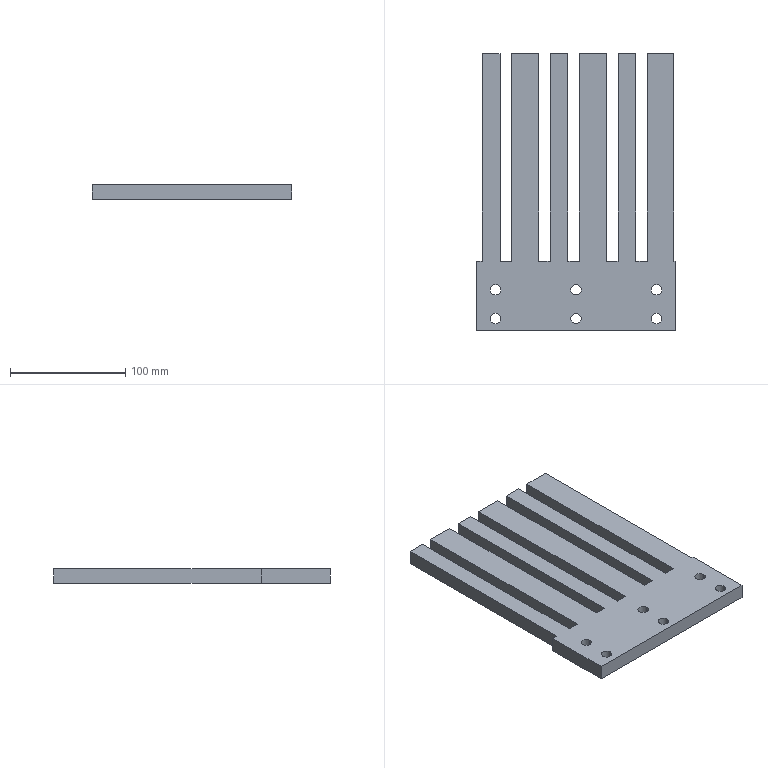Part | STEP file | 44-02-15 Press Plate | 1 solid | 42 faces | box 173 x 240 x 13 mm | volume 402588 mm3 | plane 30 | cylinder 12 | commonest cylinder face diameters 9 x12